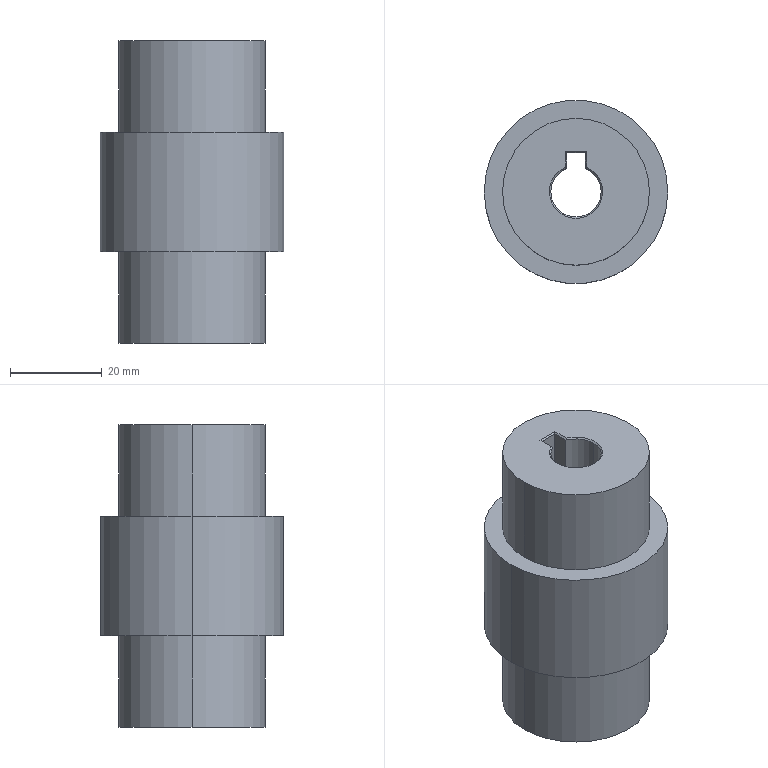Part | SolidWorks | features Cut 5, Boss 2, Chamfer 1, Extrusion 1 | 1 solid | 39 faces | box 40 x 40 x 66 mm | volume 50078 mm3 | plane 19 | cylinder 14 | cone 6 | commonest cylinder face diameters 32 x4 11 x3 19 x3 20 x2 40 x2
STEP:
#1=CARTESIAN_POINT('',(-5.5,0.,65.7));
#2=VERTEX_POINT('',#1);
#3=CARTESIAN_POINT('',(5.5,0.,65.7));
#4=VERTEX_POINT('',#3);
#5=CARTESIAN_POINT('',(0.,0.,65.7));
#6=DIRECTION('',(0.,0.,1.));
#7=DIRECTION('',(1.,0.,0.));
#8=AXIS2_PLACEMENT_3D('',#5,#6,#7);
#9=CIRCLE('',#8,5.5);
#10=EDGE_CURVE('',#2,#4,#9,.T.);
#11=ORIENTED_EDGE('',*,*,#10,.F.);
#12=CARTESIAN_POINT('',(-5.8,0.,66.));
#13=VERTEX_POINT('',#12);
#14=CARTESIAN_POINT('',(-5.5,0.,65.7));
#15=DIRECTION('',(-0.7071,0.,0.7071));
#16=VECTOR('',#15,1000.);
#17=LINE('',#14,#16);
#18=EDGE_CURVE('',#2,#13,#17,.T.);
#19=ORIENTED_EDGE('',*,*,#18,.T.);
#20=CARTESIAN_POINT('',(5.8,0.,66.));
#21=VERTEX_POINT('',#20);
#22=CARTESIAN_POINT('',(0.,0.,66.));
#23=DIRECTION('',(0.,0.,-1.));
#24=DIRECTION('',(1.,0.,0.));
#25=AXIS2_PLACEMENT_3D('',#22,#23,#24);
#26=CIRCLE('',#25,5.8);
#27=EDGE_CURVE('',#21,#13,#26,.T.);
#28=ORIENTED_EDGE('',*,*,#27,.F.);
#29=CARTESIAN_POINT('',(5.5,0.,65.7));
#30=DIRECTION('',(0.7071,0.,0.7071));
#31=VECTOR('',#30,1000.);
#32=LINE('',#29,#31);
#33=EDGE_CURVE('',#4,#21,#32,.T.);
#34=ORIENTED_EDGE('',*,*,#33,.F.);
#35=EDGE_LOOP('',(#11,#19,#28,#34));
#36=FACE_OUTER_BOUND('',#35,.T.);
#37=CARTESIAN_POINT('',(0.,0.,65.7));
#38=DIRECTION('',(0.,0.,1.));
#39=DIRECTION('',(1.,0.,0.));
#40=AXIS2_PLACEMENT_3D('',#37,#38,#39);
#41=CONICAL_SURFACE('',#40,5.5,0.7854);
#42=ADVANCED_FACE('',(#36),#41,.F.);
#43=CARTESIAN_POINT('',(2.,5.123,65.7));
#44=VERTEX_POINT('',#43);
#45=CARTESIAN_POINT('',(0.,0.,65.7));
#46=DIRECTION('',(0.,0.,1.));
#47=DIRECTION('',(1.,0.,0.));
#48=AXIS2_PLACEMENT_3D('',#45,#46,#47);
#49=CIRCLE('',#48,5.5);
#50=EDGE_CURVE('',#4,#44,#49,.T.);
#51=ORIENTED_EDGE('',*,*,#50,.F.);
#52=ORIENTED_EDGE('',*,*,#33,.T.);
#53=CARTESIAN_POINT('',(2.3,5.324,66.));
#54=VERTEX_POINT('',#53);
#55=CARTESIAN_POINT('',(0.,0.,66.));
#56=DIRECTION('',(0.,0.,-1.));
#57=DIRECTION('',(1.,0.,0.));
#58=AXIS2_PLACEMENT_3D('',#55,#56,#57);
#59=CIRCLE('',#58,5.8);
#60=EDGE_CURVE('',#54,#21,#59,.T.);
#61=ORIENTED_EDGE('',*,*,#60,.F.);
#62=CARTESIAN_POINT('',(2.,5.123,65.7));
#63=CARTESIAN_POINT('',(2.1,5.192,65.8));
#64=CARTESIAN_POINT('',(2.2,5.259,65.9));
#65=CARTESIAN_POINT('',(2.3,5.324,66.));
#66=B_SPLINE_CURVE_WITH_KNOTS('',3,(#62,#63,#64,#65),.UNSPECIFIED.,.F.,.F.,(4,4),(0.,0.0004695),.UNSPECIFIED.);
#67=EDGE_CURVE('',#44,#54,#66,.T.);
#68=ORIENTED_EDGE('',*,*,#67,.F.);
#69=EDGE_LOOP('',(#51,#52,#61,#68));
#70=FACE_OUTER_BOUND('',#69,.T.);
#71=CARTESIAN_POINT('',(0.,0.,65.7));
#72=DIRECTION('',(0.,0.,1.));
#73=DIRECTION('',(1.,0.,0.));
#74=AXIS2_PLACEMENT_3D('',#71,#72,#73);
#75=CONICAL_SURFACE('',#74,5.5,0.7854);
#76=ADVANCED_FACE('',(#70),#75,.F.);
#77=CARTESIAN_POINT('',(9.5,0.,0.3));
#78=VERTEX_POINT('',#77);
#79=CARTESIAN_POINT('',(-9.5,0.,0.3));
#80=VERTEX_POINT('',#79);
#81=CARTESIAN_POINT('',(0.,0.,0.3));
#82=DIRECTION('',(0.,0.,-1.));
#83=DIRECTION('',(1.,0.,0.));
#84=AXIS2_PLACEMENT_3D('',#81,#82,#83);
#85=CIRCLE('',#84,9.5);
#86=EDGE_CURVE('',#78,#80,#85,.T.);
#87=ORIENTED_EDGE('',*,*,#86,.F.);
#88=CARTESIAN_POINT('',(9.8,0.,0.));
#89=VERTEX_POINT('',#88);
#90=CARTESIAN_POINT('',(9.5,0.,0.3));
#91=DIRECTION('',(0.7071,0.,-0.7071));
#92=VECTOR('',#91,1000.);
#93=LINE('',#90,#92);
#94=EDGE_CURVE('',#78,#89,#93,.T.);
#95=ORIENTED_EDGE('',*,*,#94,.T.);
#96=CARTESIAN_POINT('',(-9.8,0.,0.));
#97=VERTEX_POINT('',#96);
#98=CARTESIAN_POINT('',(0.,0.,0.));
#99=DIRECTION('',(0.,0.,1.));
#100=DIRECTION('',(1.,0.,0.));
#101=AXIS2_PLACEMENT_3D('',#98,#99,#100);
#102=CIRCLE('',#101,9.8);
#103=EDGE_CURVE('',#97,#89,#102,.T.);
#104=ORIENTED_EDGE('',*,*,#103,.F.);
#105=CARTESIAN_POINT('',(-9.5,0.,0.3));
#106=DIRECTION('',(-0.7071,0.,-0.7071));
#107=VECTOR('',#106,1000.);
#108=LINE('',#105,#107);
#109=EDGE_CURVE('',#80,#97,#108,.T.);
#110=ORIENTED_EDGE('',*,*,#109,.F.);
#111=EDGE_LOOP('',(#87,#95,#104,#110));
#112=FACE_OUTER_BOUND('',#111,.T.);
#113=CARTESIAN_POINT('',(0.,0.,0.3));
#114=DIRECTION('',(0.,0.,-1.));
#115=DIRECTION('',(-1.,0.,0.));
#116=AXIS2_PLACEMENT_3D('',#113,#114,#115);
#117=CONICAL_SURFACE('',#116,9.5,0.7854);
#118=ADVANCED_FACE('',(#112),#117,.F.);
#119=CARTESIAN_POINT('',(-3.,9.014,0.3));
#120=VERTEX_POINT('',#119);
#121=CARTESIAN_POINT('',(0.,0.,0.3));
#122=DIRECTION('',(0.,0.,-1.));
#123=DIRECTION('',(1.,0.,0.));
#124=AXIS2_PLACEMENT_3D('',#121,#122,#123);
#125=CIRCLE('',#124,9.5);
#126=EDGE_CURVE('',#80,#120,#125,.T.);
#127=ORIENTED_EDGE('',*,*,#126,.F.);
#128=ORIENTED_EDGE('',*,*,#109,.T.);
#129=CARTESIAN_POINT('',(-3.3,9.228,0.));
#130=VERTEX_POINT('',#129);
#131=CARTESIAN_POINT('',(0.,0.,0.));
#132=DIRECTION('',(0.,0.,1.));
#133=DIRECTION('',(1.,0.,0.));
#134=AXIS2_PLACEMENT_3D('',#131,#132,#133);
#135=CIRCLE('',#134,9.8);
#136=EDGE_CURVE('',#130,#97,#135,.T.);
#137=ORIENTED_EDGE('',*,*,#136,.F.);
#138=CARTESIAN_POINT('',(-3.,9.014,0.3));
#139=CARTESIAN_POINT('',(-3.1,9.086,0.2002));
#140=CARTESIAN_POINT('',(-3.2,9.157,0.1002));
#141=CARTESIAN_POINT('',(-3.3,9.228,0.));
#142=B_SPLINE_CURVE_WITH_KNOTS('',3,(#138,#139,#140,#141),.UNSPECIFIED.,.F.,.F.,(4,4),(0.,0.0004751),.UNSPECIFIED.);
#143=EDGE_CURVE('',#120,#130,#142,.T.);
#144=ORIENTED_EDGE('',*,*,#143,.F.);
#145=EDGE_LOOP('',(#127,#128,#137,#144));
#146=FACE_OUTER_BOUND('',#145,.T.);
#147=CARTESIAN_POINT('',(0.,0.,0.3));
#148=DIRECTION('',(0.,0.,-1.));
#149=DIRECTION('',(-1.,0.,0.));
#150=AXIS2_PLACEMENT_3D('',#147,#148,#149);
#151=CONICAL_SURFACE('',#150,9.5,0.7854);
#152=ADVANCED_FACE('',(#146),#151,.F.);
#153=CARTESIAN_POINT('',(-10.,0.,27.));
#154=VERTEX_POINT('',#153);
#155=CARTESIAN_POINT('',(10.,0.,27.));
#156=VERTEX_POINT('',#155);
#157=CARTESIAN_POINT('',(0.,0.,27.));
#158=DIRECTION('',(0.,0.,1.));
#159=DIRECTION('',(1.,0.,0.));
#160=AXIS2_PLACEMENT_3D('',#157,#158,#159);
#161=CIRCLE('',#160,10.);
#162=EDGE_CURVE('',#154,#156,#161,.T.);
#163=ORIENTED_EDGE('',*,*,#162,.F.);
#164=CARTESIAN_POINT('',(-10.,0.,39.));
#165=VERTEX_POINT('',#164);
#166=CARTESIAN_POINT('',(-10.,0.,27.));
#167=DIRECTION('',(0.,0.,1.));
#168=VECTOR('',#167,1000.);
#169=LINE('',#166,#168);
#170=EDGE_CURVE('',#154,#165,#169,.T.);
#171=ORIENTED_EDGE('',*,*,#170,.T.);
#172=CARTESIAN_POINT('',(10.,0.,39.));
#173=VERTEX_POINT('',#172);
#174=CARTESIAN_POINT('',(0.,0.,39.));
#175=DIRECTION('',(0.,0.,1.));
#176=DIRECTION('',(1.,0.,0.));
#177=AXIS2_PLACEMENT_3D('',#174,#175,#176);
#178=CIRCLE('',#177,10.);
#179=EDGE_CURVE('',#165,#173,#178,.T.);
#180=ORIENTED_EDGE('',*,*,#179,.T.);
#181=CARTESIAN_POINT('',(10.,0.,27.));
#182=DIRECTION('',(0.,0.,1.));
#183=VECTOR('',#182,1000.);
#184=LINE('',#181,#183);
#185=EDGE_CURVE('',#156,#173,#184,.T.);
#186=ORIENTED_EDGE('',*,*,#185,.F.);
#187=EDGE_LOOP('',(#163,#171,#180,#186));
#188=FACE_OUTER_BOUND('',#187,.T.);
#189=CARTESIAN_POINT('',(0.,0.,27.));
#190=DIRECTION('',(0.,0.,1.));
#191=DIRECTION('',(1.,0.,0.));
#192=AXIS2_PLACEMENT_3D('',#189,#190,#191);
#193=CYLINDRICAL_SURFACE('',#192,10.);
#194=ADVANCED_FACE('',(#188),#193,.F.);
#195=CARTESIAN_POINT('',(5.5,0.,39.));
#196=VERTEX_POINT('',#195);
#197=CARTESIAN_POINT('',(-5.5,0.,39.));
#198=VERTEX_POINT('',#197);
#199=CARTESIAN_POINT('',(0.,0.,39.));
#200=DIRECTION('',(0.,0.,-1.));
#201=DIRECTION('',(1.,0.,0.));
#202=AXIS2_PLACEMENT_3D('',#199,#200,#201);
#203=CIRCLE('',#202,5.5);
#204=EDGE_CURVE('',#196,#198,#203,.T.);
#205=ORIENTED_EDGE('',*,*,#204,.T.);
#206=CARTESIAN_POINT('',(-5.5,0.,39.));
#207=DIRECTION('',(0.,0.,1.));
#208=VECTOR('',#207,1000.);
#209=LINE('',#206,#208);
#210=EDGE_CURVE('',#198,#2,#209,.T.);
#211=ORIENTED_EDGE('',*,*,#210,.T.);
#212=ORIENTED_EDGE('',*,*,#10,.T.);
#213=CARTESIAN_POINT('',(5.5,0.,39.));
#214=DIRECTION('',(0.,0.,1.));
#215=VECTOR('',#214,1000.);
#216=LINE('',#213,#215);
#217=EDGE_CURVE('',#196,#4,#216,.T.);
#218=ORIENTED_EDGE('',*,*,#217,.F.);
#219=EDGE_LOOP('',(#205,#211,#212,#218));
#220=FACE_OUTER_BOUND('',#219,.T.);
#221=CARTESIAN_POINT('',(0.,0.,39.));
#222=DIRECTION('',(0.,0.,1.));
#223=DIRECTION('',(1.,0.,0.));
#224=AXIS2_PLACEMENT_3D('',#221,#222,#223);
#225=CYLINDRICAL_SURFACE('',#224,5.5);
#226=ADVANCED_FACE('',(#220),#225,.F.);
#227=CARTESIAN_POINT('',(2.,5.123,39.));
#228=VERTEX_POINT('',#227);
#229=CARTESIAN_POINT('',(0.,0.,39.));
#230=DIRECTION('',(0.,0.,-1.));
#231=DIRECTION('',(1.,0.,0.));
#232=AXIS2_PLACEMENT_3D('',#229,#230,#231);
#233=CIRCLE('',#232,5.5);
#234=EDGE_CURVE('',#228,#196,#233,.T.);
#235=ORIENTED_EDGE('',*,*,#234,.T.);
#236=ORIENTED_EDGE('',*,*,#217,.T.);
#237=ORIENTED_EDGE('',*,*,#50,.T.);
#238=CARTESIAN_POINT('',(2.,5.123,39.));
#239=DIRECTION('',(0.,0.,1.));
#240=VECTOR('',#239,1000.);
#241=LINE('',#238,#240);
#242=EDGE_CURVE('',#228,#44,#241,.T.);
#243=ORIENTED_EDGE('',*,*,#242,.F.);
#244=EDGE_LOOP('',(#235,#236,#237,#243));
#245=FACE_OUTER_BOUND('',#244,.T.);
#246=CARTESIAN_POINT('',(0.,0.,39.));
#247=DIRECTION('',(0.,0.,1.));
#248=DIRECTION('',(1.,0.,0.));
#249=AXIS2_PLACEMENT_3D('',#246,#247,#248);
#250=CYLINDRICAL_SURFACE('',#249,5.5);
#251=ADVANCED_FACE('',(#245),#250,.F.);
#252=CARTESIAN_POINT('',(9.5,0.,27.));
#253=VERTEX_POINT('',#252);
#254=CARTESIAN_POINT('',(-9.5,0.,27.));
#255=VERTEX_POINT('',#254);
#256=CARTESIAN_POINT('',(0.,0.,27.));
#257=DIRECTION('',(0.,0.,-1.));
#258=DIRECTION('',(1.,0.,0.));
#259=AXIS2_PLACEMENT_3D('',#256,#257,#258);
#260=CIRCLE('',#259,9.5);
#261=EDGE_CURVE('',#253,#255,#260,.T.);
#262=ORIENTED_EDGE('',*,*,#261,.F.);
#263=CARTESIAN_POINT('',(9.5,0.,27.));
#264=DIRECTION('',(0.,0.,-1.));
#265=VECTOR('',#264,1000.);
#266=LINE('',#263,#265);
#267=EDGE_CURVE('',#253,#78,#266,.T.);
#268=ORIENTED_EDGE('',*,*,#267,.T.);
#269=ORIENTED_EDGE('',*,*,#86,.T.);
#270=CARTESIAN_POINT('',(-9.5,0.,27.));
#271=DIRECTION('',(0.,0.,-1.));
#272=VECTOR('',#271,1000.);
#273=LINE('',#270,#272);
#274=EDGE_CURVE('',#255,#80,#273,.T.);
#275=ORIENTED_EDGE('',*,*,#274,.F.);
#276=EDGE_LOOP('',(#262,#268,#269,#275));
#277=FACE_OUTER_BOUND('',#276,.T.);
#278=CARTESIAN_POINT('',(0.,0.,27.));
#279=DIRECTION('',(0.,0.,-1.));
#280=DIRECTION('',(-1.,0.,0.));
#281=AXIS2_PLACEMENT_3D('',#278,#279,#280);
#282=CYLINDRICAL_SURFACE('',#281,9.5);
#283=ADVANCED_FACE('',(#277),#282,.F.);
#284=CARTESIAN_POINT('',(-3.,9.014,27.));
#285=VERTEX_POINT('',#284);
#286=CARTESIAN_POINT('',(0.,0.,27.));
#287=DIRECTION('',(0.,0.,-1.));
#288=DIRECTION('',(1.,0.,0.));
#289=AXIS2_PLACEMENT_3D('',#286,#287,#288);
#290=CIRCLE('',#289,9.5);
#291=EDGE_CURVE('',#255,#285,#290,.T.);
#292=ORIENTED_EDGE('',*,*,#291,.F.);
#293=ORIENTED_EDGE('',*,*,#274,.T.);
#294=ORIENTED_EDGE('',*,*,#126,.T.);
#295=CARTESIAN_POINT('',(-3.,9.014,27.));
#296=DIRECTION('',(0.,0.,-1.));
#297=VECTOR('',#296,1000.);
#298=LINE('',#295,#297);
#299=EDGE_CURVE('',#285,#120,#298,.T.);
#300=ORIENTED_EDGE('',*,*,#299,.F.);
#301=EDGE_LOOP('',(#292,#293,#294,#300));
#302=FACE_OUTER_BOUND('',#301,.T.);
#303=CARTESIAN_POINT('',(0.,0.,27.));
#304=DIRECTION('',(0.,0.,-1.));
#305=DIRECTION('',(-1.,0.,0.));
#306=AXIS2_PLACEMENT_3D('',#303,#304,#305);
#307=CYLINDRICAL_SURFACE('',#306,9.5);
#308=ADVANCED_FACE('',(#302),#307,.F.);
#309=CARTESIAN_POINT('',(16.,0.,66.));
#310=VERTEX_POINT('',#309);
#311=CARTESIAN_POINT('',(-16.,0.,66.));
#312=VERTEX_POINT('',#311);
#313=CARTESIAN_POINT('',(0.,0.,66.));
#314=DIRECTION('',(0.,0.,1.));
#315=DIRECTION('',(1.,0.,0.));
#316=AXIS2_PLACEMENT_3D('',#313,#314,#315);
#317=CIRCLE('',#316,16.);
#318=EDGE_CURVE('',#310,#312,#317,.T.);
#319=ORIENTED_EDGE('',*,*,#318,.F.);
#320=CARTESIAN_POINT('',(16.,0.,46.));
#321=VERTEX_POINT('',#320);
#322=CARTESIAN_POINT('',(16.,0.,66.));
#323=DIRECTION('',(0.,0.,-1.));
#324=VECTOR('',#323,1000.);
#325=LINE('',#322,#324);
#326=EDGE_CURVE('',#310,#321,#325,.T.);
#327=ORIENTED_EDGE('',*,*,#326,.T.);
#328=CARTESIAN_POINT('',(-16.,0.,46.));
#329=VERTEX_POINT('',#328);
#330=CARTESIAN_POINT('',(0.,0.,46.));
#331=DIRECTION('',(0.,0.,1.));
#332=DIRECTION('',(1.,0.,0.));
#333=AXIS2_PLACEMENT_3D('',#330,#331,#332);
#334=CIRCLE('',#333,16.);
#335=EDGE_CURVE('',#321,#329,#334,.T.);
#336=ORIENTED_EDGE('',*,*,#335,.T.);
#337=CARTESIAN_POINT('',(-16.,0.,66.));
#338=DIRECTION('',(0.,0.,-1.));
#339=VECTOR('',#338,1000.);
#340=LINE('',#337,#339);
#341=EDGE_CURVE('',#312,#329,#340,.T.);
#342=ORIENTED_EDGE('',*,*,#341,.F.);
#343=EDGE_LOOP('',(#319,#327,#336,#342));
#344=FACE_OUTER_BOUND('',#343,.T.);
#345=CARTESIAN_POINT('',(0.,0.,66.));
#346=DIRECTION('',(0.,0.,-1.));
#347=DIRECTION('',(-1.,0.,0.));
#348=AXIS2_PLACEMENT_3D('',#345,#346,#347);
#349=CYLINDRICAL_SURFACE('',#348,16.);
#350=ADVANCED_FACE('',(#344),#349,.T.);
#351=CARTESIAN_POINT('',(20.,0.,46.));
#352=VERTEX_POINT('',#351);
#353=CARTESIAN_POINT('',(-20.,0.,46.));
#354=VERTEX_POINT('',#353);
#355=CARTESIAN_POINT('',(0.,0.,46.));
#356=DIRECTION('',(0.,0.,1.));
#357=DIRECTION('',(1.,0.,0.));
#358=AXIS2_PLACEMENT_3D('',#355,#356,#357);
#359=CIRCLE('',#358,20.);
#360=EDGE_CURVE('',#352,#354,#359,.T.);
#361=ORIENTED_EDGE('',*,*,#360,.F.);
#362=CARTESIAN_POINT('',(20.,0.,20.));
#363=VERTEX_POINT('',#362);
#364=CARTESIAN_POINT('',(20.,0.,46.));
#365=DIRECTION('',(0.,0.,-1.));
#366=VECTOR('',#365,1000.);
#367=LINE('',#364,#366);
#368=EDGE_CURVE('',#352,#363,#367,.T.);
#369=ORIENTED_EDGE('',*,*,#368,.T.);
#370=CARTESIAN_POINT('',(-20.,0.,20.));
#371=VERTEX_POINT('',#370);
#372=CARTESIAN_POINT('',(0.,0.,20.));
#373=DIRECTION('',(0.,0.,1.));
#374=DIRECTION('',(1.,0.,0.));
#375=AXIS2_PLACEMENT_3D('',#372,#373,#374);
#376=CIRCLE('',#375,20.);
#377=EDGE_CURVE('',#363,#371,#376,.T.);
#378=ORIENTED_EDGE('',*,*,#377,.T.);
#379=CARTESIAN_POINT('',(-20.,0.,46.));
#380=DIRECTION('',(0.,0.,-1.));
#381=VECTOR('',#380,1000.);
#382=LINE('',#379,#381);
#383=EDGE_CURVE('',#354,#371,#382,.T.);
#384=ORIENTED_EDGE('',*,*,#383,.F.);
#385=EDGE_LOOP('',(#361,#369,#378,#384));
#386=FACE_OUTER_BOUND('',#385,.T.);
#387=CARTESIAN_POINT('',(0.,0.,46.));
#388=DIRECTION('',(0.,0.,-1.));
#389=DIRECTION('',(-1.,0.,0.));
#390=AXIS2_PLACEMENT_3D('',#387,#388,#389);
#391=CYLINDRICAL_SURFACE('',#390,20.);
#392=ADVANCED_FACE('',(#386),#391,.T.);
#393=CARTESIAN_POINT('',(16.,0.,20.));
#394=VERTEX_POINT('',#393);
#395=CARTESIAN_POINT('',(-16.,0.,20.));
#396=VERTEX_POINT('',#395);
#397=CARTESIAN_POINT('',(0.,0.,20.));
#398=DIRECTION('',(0.,0.,1.));
#399=DIRECTION('',(1.,0.,0.));
#400=AXIS2_PLACEMENT_3D('',#397,#398,#399);
#401=CIRCLE('',#400,16.);
#402=EDGE_CURVE('',#394,#396,#401,.T.);
#403=ORIENTED_EDGE('',*,*,#402,.F.);
#404=CARTESIAN_POINT('',(16.,0.,0.));
#405=VERTEX_POINT('',#404);
#406=CARTESIAN_POINT('',(16.,0.,20.));
#407=DIRECTION('',(0.,0.,-1.));
#408=VECTOR('',#407,1000.);
#409=LINE('',#406,#408);
#410=EDGE_CURVE('',#394,#405,#409,.T.);
#411=ORIENTED_EDGE('',*,*,#410,.T.);
#412=CARTESIAN_POINT('',(-16.,0.,0.));
#413=VERTEX_POINT('',#412);
#414=CARTESIAN_POINT('',(0.,0.,0.));
#415=DIRECTION('',(0.,0.,1.));
#416=DIRECTION('',(1.,0.,0.));
#417=AXIS2_PLACEMENT_3D('',#414,#415,#416);
#418=CIRCLE('',#417,16.);
#419=EDGE_CURVE('',#405,#413,#418,.T.);
#420=ORIENTED_EDGE('',*,*,#419,.T.);
#421=CARTESIAN_POINT('',(-16.,0.,20.));
#422=DIRECTION('',(0.,0.,-1.));
#423=VECTOR('',#422,1000.);
#424=LINE('',#421,#423);
#425=EDGE_CURVE('',#396,#413,#424,.T.);
#426=ORIENTED_EDGE('',*,*,#425,.F.);
#427=EDGE_LOOP('',(#403,#411,#420,#426));
#428=FACE_OUTER_BOUND('',#427,.T.);
#429=CARTESIAN_POINT('',(0.,0.,20.));
#430=DIRECTION('',(0.,0.,-1.));
#431=DIRECTION('',(-1.,0.,0.));
#432=AXIS2_PLACEMENT_3D('',#429,#430,#431);
#433=CYLINDRICAL_SURFACE('',#432,16.);
#434=ADVANCED_FACE('',(#428),#433,.T.);
#435=CARTESIAN_POINT('',(0.,0.,46.));
#436=DIRECTION('',(0.,0.,1.));
#437=DIRECTION('',(1.,0.,0.));
#438=AXIS2_PLACEMENT_3D('',#435,#436,#437);
#439=CIRCLE('',#438,20.);
#440=EDGE_CURVE('',#354,#352,#439,.T.);
#441=ORIENTED_EDGE('',*,*,#440,.T.);
#442=ORIENTED_EDGE('',*,*,#360,.T.);
#443=EDGE_LOOP('',(#441,#442));
#444=FACE_OUTER_BOUND('',#443,.T.);
#445=CARTESIAN_POINT('',(0.,0.,46.));
#446=DIRECTION('',(0.,0.,1.));
#447=DIRECTION('',(1.,0.,0.));
#448=AXIS2_PLACEMENT_3D('',#445,#446,#447);
#449=CIRCLE('',#448,16.);
#450=EDGE_CURVE('',#329,#321,#449,.T.);
#451=ORIENTED_EDGE('',*,*,#450,.F.);
#452=ORIENTED_EDGE('',*,*,#335,.F.);
#453=EDGE_LOOP('',(#451,#452));
#454=FACE_BOUND('',#453,.T.);
#455=CARTESIAN_POINT('',(0.,0.,46.));
#456=DIRECTION('',(0.,0.,1.));
#457=DIRECTION('',(1.,0.,0.));
#458=AXIS2_PLACEMENT_3D('',#455,#456,#457);
#459=PLANE('',#458);
#460=ADVANCED_FACE('',(#444,#454),#459,.T.);
#461=ORIENTED_EDGE('',*,*,#410,.F.);
#462=CARTESIAN_POINT('',(0.,0.,20.));
#463=DIRECTION('',(0.,0.,1.));
#464=DIRECTION('',(1.,0.,0.));
#465=AXIS2_PLACEMENT_3D('',#462,#463,#464);
#466=CIRCLE('',#465,16.);
#467=EDGE_CURVE('',#396,#394,#466,.T.);
#468=ORIENTED_EDGE('',*,*,#467,.F.);
#469=ORIENTED_EDGE('',*,*,#425,.T.);
#470=CARTESIAN_POINT('',(0.,0.,0.));
#471=DIRECTION('',(0.,0.,1.));
#472=DIRECTION('',(1.,0.,0.));
#473=AXIS2_PLACEMENT_3D('',#470,#471,#472);
#474=CIRCLE('',#473,16.);
#475=EDGE_CURVE('',#413,#405,#474,.T.);
#476=ORIENTED_EDGE('',*,*,#475,.T.);
#477=EDGE_LOOP('',(#461,#468,#469,#476));
#478=FACE_OUTER_BOUND('',#477,.T.);
#479=CARTESIAN_POINT('',(0.,0.,20.));
#480=DIRECTION('',(0.,0.,-1.));
#481=DIRECTION('',(-1.,0.,0.));
#482=AXIS2_PLACEMENT_3D('',#479,#480,#481);
#483=CYLINDRICAL_SURFACE('',#482,16.);
#484=ADVANCED_FACE('',(#478),#483,.T.);
#485=CARTESIAN_POINT('',(3.3,12.3,0.));
#486=VERTEX_POINT('',#485);
#487=CARTESIAN_POINT('',(-3.3,12.3,0.));
#488=VERTEX_POINT('',#487);
#489=CARTESIAN_POINT('',(0.,12.3,0.));
#490=DIRECTION('',(-1.,0.,0.));
#491=VECTOR('',#490,1000.);
#492=LINE('',#489,#491);
#493=EDGE_CURVE('',#486,#488,#492,.T.);
#494=ORIENTED_EDGE('',*,*,#493,.T.);
#495=CARTESIAN_POINT('',(-3.3,0.,0.));
#496=DIRECTION('',(0.,-1.,0.));
#497=VECTOR('',#496,1000.);
#498=LINE('',#495,#497);
#499=EDGE_CURVE('',#488,#130,#498,.T.);
#500=ORIENTED_EDGE('',*,*,#499,.T.);
#501=ORIENTED_EDGE('',*,*,#136,.T.);
#502=ORIENTED_EDGE('',*,*,#103,.T.);
#503=CARTESIAN_POINT('',(3.3,9.228,0.));
#504=VERTEX_POINT('',#503);
#505=CARTESIAN_POINT('',(0.,0.,0.));
#506=DIRECTION('',(0.,0.,1.));
#507=DIRECTION('',(1.,0.,0.));
#508=AXIS2_PLACEMENT_3D('',#505,#506,#507);
#509=CIRCLE('',#508,9.8);
#510=EDGE_CURVE('',#89,#504,#509,.T.);
#511=ORIENTED_EDGE('',*,*,#510,.T.);
#512=CARTESIAN_POINT('',(3.3,0.,0.));
#513=DIRECTION('',(0.,1.,0.));
#514=VECTOR('',#513,1000.);
#515=LINE('',#512,#514);
#516=EDGE_CURVE('',#504,#486,#515,.T.);
#517=ORIENTED_EDGE('',*,*,#516,.T.);
#518=EDGE_LOOP('',(#494,#500,#501,#502,#511,#517));
#519=FACE_BOUND('',#518,.T.);
#520=ORIENTED_EDGE('',*,*,#475,.F.);
#521=ORIENTED_EDGE('',*,*,#419,.F.);
#522=EDGE_LOOP('',(#520,#521));
#523=FACE_OUTER_BOUND('',#522,.T.);
#524=CARTESIAN_POINT('',(0.,0.,0.));
#525=DIRECTION('',(0.,0.,1.));
#526=DIRECTION('',(1.,0.,0.));
#527=AXIS2_PLACEMENT_3D('',#524,#525,#526);
#528=PLANE('',#527);
#529=ADVANCED_FACE('',(#519,#523),#528,.F.);
#530=CARTESIAN_POINT('',(0.,0.,20.));
#531=DIRECTION('',(0.,0.,1.));
#532=DIRECTION('',(1.,0.,0.));
#533=AXIS2_PLACEMENT_3D('',#530,#531,#532);
#534=CIRCLE('',#533,20.);
#535=EDGE_CURVE('',#371,#363,#534,.T.);
#536=ORIENTED_EDGE('',*,*,#535,.F.);
#537=ORIENTED_EDGE('',*,*,#377,.F.);
#538=EDGE_LOOP('',(#536,#537));
#539=FACE_OUTER_BOUND('',#538,.T.);
#540=ORIENTED_EDGE('',*,*,#467,.T.);
#541=ORIENTED_EDGE('',*,*,#402,.T.);
#542=EDGE_LOOP('',(#540,#541));
#543=FACE_BOUND('',#542,.T.);
#544=CARTESIAN_POINT('',(0.,0.,20.));
#545=DIRECTION('',(0.,0.,1.));
#546=DIRECTION('',(1.,0.,0.));
#547=AXIS2_PLACEMENT_3D('',#544,#545,#546);
#548=PLANE('',#547);
#549=ADVANCED_FACE('',(#539,#543),#548,.F.);
#550=ORIENTED_EDGE('',*,*,#368,.F.);
#551=ORIENTED_EDGE('',*,*,#440,.F.);
#552=ORIENTED_EDGE('',*,*,#383,.T.);
#553=ORIENTED_EDGE('',*,*,#535,.T.);
#554=EDGE_LOOP('',(#550,#551,#552,#553));
#555=FACE_OUTER_BOUND('',#554,.T.);
#556=CARTESIAN_POINT('',(0.,0.,46.));
#557=DIRECTION('',(0.,0.,-1.));
#558=DIRECTION('',(-1.,0.,0.));
#559=AXIS2_PLACEMENT_3D('',#556,#557,#558);
#560=CYLINDRICAL_SURFACE('',#559,20.);
#561=ADVANCED_FACE('',(#555),#560,.T.);
#562=ORIENTED_EDGE('',*,*,#326,.F.);
#563=CARTESIAN_POINT('',(0.,0.,66.));
#564=DIRECTION('',(0.,0.,1.));
#565=DIRECTION('',(1.,0.,0.));
#566=AXIS2_PLACEMENT_3D('',#563,#564,#565);
#567=CIRCLE('',#566,16.);
#568=EDGE_CURVE('',#312,#310,#567,.T.);
#569=ORIENTED_EDGE('',*,*,#568,.F.);
#570=ORIENTED_EDGE('',*,*,#341,.T.);
#571=ORIENTED_EDGE('',*,*,#450,.T.);
#572=EDGE_LOOP('',(#562,#569,#570,#571));
#573=FACE_OUTER_BOUND('',#572,.T.);
#574=CARTESIAN_POINT('',(0.,0.,66.));
#575=DIRECTION('',(0.,0.,-1.));
#576=DIRECTION('',(-1.,0.,0.));
#577=AXIS2_PLACEMENT_3D('',#574,#575,#576);
#578=CYLINDRICAL_SURFACE('',#577,16.);
#579=ADVANCED_FACE('',(#573),#578,.T.);
#580=CARTESIAN_POINT('',(-2.3,8.8,66.));
#581=VERTEX_POINT('',#580);
#582=CARTESIAN_POINT('',(2.3,8.8,66.));
#583=VERTEX_POINT('',#582);
#584=CARTESIAN_POINT('',(2.,8.8,66.));
#585=DIRECTION('',(1.,0.,0.));
#586=VECTOR('',#585,1000.);
#587=LINE('',#584,#586);
#588=EDGE_CURVE('',#581,#583,#587,.T.);
#589=ORIENTED_EDGE('',*,*,#588,.T.);
#590=CARTESIAN_POINT('',(2.3,5.123,66.));
#591=DIRECTION('',(0.,-1.,0.));
#592=VECTOR('',#591,1000.);
#593=LINE('',#590,#592);
#594=EDGE_CURVE('',#583,#54,#593,.T.);
#595=ORIENTED_EDGE('',*,*,#594,.T.);
#596=ORIENTED_EDGE('',*,*,#60,.T.);
#597=ORIENTED_EDGE('',*,*,#27,.T.);
#598=CARTESIAN_POINT('',(-2.3,5.324,66.));
#599=VERTEX_POINT('',#598);
#600=CARTESIAN_POINT('',(0.,0.,66.));
#601=DIRECTION('',(0.,0.,-1.));
#602=DIRECTION('',(1.,0.,0.));
#603=AXIS2_PLACEMENT_3D('',#600,#601,#602);
#604=CIRCLE('',#603,5.8);
#605=EDGE_CURVE('',#13,#599,#604,.T.);
#606=ORIENTED_EDGE('',*,*,#605,.T.);
#607=CARTESIAN_POINT('',(-2.3,8.5,66.));
#608=DIRECTION('',(0.,1.,0.));
#609=VECTOR('',#608,1000.);
#610=LINE('',#607,#609);
#611=EDGE_CURVE('',#599,#581,#610,.T.);
#612=ORIENTED_EDGE('',*,*,#611,.T.);
#613=EDGE_LOOP('',(#589,#595,#596,#597,#606,#612));
#614=FACE_BOUND('',#613,.T.);
#615=ORIENTED_EDGE('',*,*,#568,.T.);
#616=ORIENTED_EDGE('',*,*,#318,.T.);
#617=EDGE_LOOP('',(#615,#616));
#618=FACE_OUTER_BOUND('',#617,.T.);
#619=CARTESIAN_POINT('',(0.,0.,66.));
#620=DIRECTION('',(0.,0.,1.));
#621=DIRECTION('',(1.,0.,0.));
#622=AXIS2_PLACEMENT_3D('',#619,#620,#621);
#623=PLANE('',#622);
#624=ADVANCED_FACE('',(#614,#618),#623,.T.);
#625=ORIENTED_EDGE('',*,*,#267,.F.);
#626=CARTESIAN_POINT('',(3.,9.014,27.));
#627=VERTEX_POINT('',#626);
#628=CARTESIAN_POINT('',(0.,0.,27.));
#629=DIRECTION('',(0.,0.,-1.));
#630=DIRECTION('',(1.,0.,0.));
#631=AXIS2_PLACEMENT_3D('',#628,#629,#630);
#632=CIRCLE('',#631,9.5);
#633=EDGE_CURVE('',#627,#253,#632,.T.);
#634=ORIENTED_EDGE('',*,*,#633,.F.);
#635=CARTESIAN_POINT('',(3.,9.014,0.3));
#636=VERTEX_POINT('',#635);
#637=CARTESIAN_POINT('',(3.,9.014,27.));
#638=DIRECTION('',(0.,0.,-1.));
#639=VECTOR('',#638,1000.);
#640=LINE('',#637,#639);
#641=EDGE_CURVE('',#627,#636,#640,.T.);
#642=ORIENTED_EDGE('',*,*,#641,.T.);
#643=CARTESIAN_POINT('',(0.,0.,0.3));
#644=DIRECTION('',(0.,0.,-1.));
#645=DIRECTION('',(1.,0.,0.));
#646=AXIS2_PLACEMENT_3D('',#643,#644,#645);
#647=CIRCLE('',#646,9.5);
#648=EDGE_CURVE('',#636,#78,#647,.T.);
#649=ORIENTED_EDGE('',*,*,#648,.T.);
#650=EDGE_LOOP('',(#625,#634,#642,#649));
#651=FACE_OUTER_BOUND('',#650,.T.);
#652=CARTESIAN_POINT('',(0.,0.,27.));
#653=DIRECTION('',(0.,0.,-1.));
#654=DIRECTION('',(-1.,0.,0.));
#655=AXIS2_PLACEMENT_3D('',#652,#653,#654);
#656=CYLINDRICAL_SURFACE('',#655,9.5);
#657=ADVANCED_FACE('',(#651),#656,.F.);
#658=ORIENTED_EDGE('',*,*,#210,.F.);
#659=CARTESIAN_POINT('',(-2.,5.123,39.));
#660=VERTEX_POINT('',#659);
#661=CARTESIAN_POINT('',(0.,0.,39.));
#662=DIRECTION('',(0.,0.,-1.));
#663=DIRECTION('',(1.,0.,0.));
#664=AXIS2_PLACEMENT_3D('',#661,#662,#663);
#665=CIRCLE('',#664,5.5);
#666=EDGE_CURVE('',#198,#660,#665,.T.);
#667=ORIENTED_EDGE('',*,*,#666,.T.);
#668=CARTESIAN_POINT('',(-2.,5.123,65.7));
#669=VERTEX_POINT('',#668);
#670=CARTESIAN_POINT('',(-2.,5.123,39.));
#671=DIRECTION('',(0.,0.,1.));
#672=VECTOR('',#671,1000.);
#673=LINE('',#670,#672);
#674=EDGE_CURVE('',#660,#669,#673,.T.);
#675=ORIENTED_EDGE('',*,*,#674,.T.);
#676=CARTESIAN_POINT('',(0.,0.,65.7));
#677=DIRECTION('',(0.,0.,1.));
#678=DIRECTION('',(1.,0.,0.));
#679=AXIS2_PLACEMENT_3D('',#676,#677,#678);
#680=CIRCLE('',#679,5.5);
#681=EDGE_CURVE('',#669,#2,#680,.T.);
#682=ORIENTED_EDGE('',*,*,#681,.T.);
#683=EDGE_LOOP('',(#658,#667,#675,#682));
#684=FACE_OUTER_BOUND('',#683,.T.);
#685=CARTESIAN_POINT('',(0.,0.,39.));
#686=DIRECTION('',(0.,0.,1.));
#687=DIRECTION('',(1.,0.,0.));
#688=AXIS2_PLACEMENT_3D('',#685,#686,#687);
#689=CYLINDRICAL_SURFACE('',#688,5.5);
#690=ADVANCED_FACE('',(#684),#689,.F.);
#691=CARTESIAN_POINT('',(-3.,9.539,27.));
#692=VERTEX_POINT('',#691);
#693=CARTESIAN_POINT('',(-3.,12.,27.));
#694=DIRECTION('',(0.,1.,0.));
#695=VECTOR('',#694,1000.);
#696=LINE('',#693,#695);
#697=EDGE_CURVE('',#285,#692,#696,.T.);
#698=ORIENTED_EDGE('',*,*,#697,.T.);
#699=CARTESIAN_POINT('',(0.,0.,27.));
#700=DIRECTION('',(0.,0.,1.));
#701=DIRECTION('',(1.,0.,0.));
#702=AXIS2_PLACEMENT_3D('',#699,#700,#701);
#703=CIRCLE('',#702,10.);
#704=EDGE_CURVE('',#692,#154,#703,.T.);
#705=ORIENTED_EDGE('',*,*,#704,.T.);
#706=ORIENTED_EDGE('',*,*,#162,.T.);
#707=CARTESIAN_POINT('',(3.,9.539,27.));
#708=VERTEX_POINT('',#707);
#709=CARTESIAN_POINT('',(0.,0.,27.));
#710=DIRECTION('',(0.,0.,1.));
#711=DIRECTION('',(1.,0.,0.));
#712=AXIS2_PLACEMENT_3D('',#709,#710,#711);
#713=CIRCLE('',#712,10.);
#714=EDGE_CURVE('',#156,#708,#713,.T.);
#715=ORIENTED_EDGE('',*,*,#714,.T.);
#716=CARTESIAN_POINT('',(3.,12.,27.));
#717=DIRECTION('',(0.,-1.,0.));
#718=VECTOR('',#717,1000.);
#719=LINE('',#716,#718);
#720=EDGE_CURVE('',#708,#627,#719,.T.);
#721=ORIENTED_EDGE('',*,*,#720,.T.);
#722=ORIENTED_EDGE('',*,*,#633,.T.);
#723=ORIENTED_EDGE('',*,*,#261,.T.);
#724=ORIENTED_EDGE('',*,*,#291,.T.);
#725=EDGE_LOOP('',(#698,#705,#706,#715,#721,#722,#723,#724));
#726=FACE_OUTER_BOUND('',#725,.T.);
#727=CARTESIAN_POINT('',(0.,0.,27.));
#728=DIRECTION('',(0.,0.,1.));
#729=DIRECTION('',(1.,0.,0.));
#730=AXIS2_PLACEMENT_3D('',#727,#728,#729);
#731=PLANE('',#730);
#732=ADVANCED_FACE('',(#726),#731,.T.);
#733=CARTESIAN_POINT('',(0.,0.,39.));
#734=DIRECTION('',(0.,0.,1.));
#735=DIRECTION('',(1.,0.,0.));
#736=AXIS2_PLACEMENT_3D('',#733,#734,#735);
#737=CIRCLE('',#736,10.);
#738=EDGE_CURVE('',#173,#165,#737,.T.);
#739=ORIENTED_EDGE('',*,*,#738,.F.);
#740=ORIENTED_EDGE('',*,*,#179,.F.);
#741=EDGE_LOOP('',(#739,#740));
#742=FACE_OUTER_BOUND('',#741,.T.);
#743=ORIENTED_EDGE('',*,*,#234,.F.);
#744=CARTESIAN_POINT('',(2.,8.5,39.));
#745=VERTEX_POINT('',#744);
#746=CARTESIAN_POINT('',(2.,8.5,39.));
#747=DIRECTION('',(0.,1.,0.));
#748=VECTOR('',#747,1000.);
#749=LINE('',#746,#748);
#750=EDGE_CURVE('',#228,#745,#749,.T.);
#751=ORIENTED_EDGE('',*,*,#750,.T.);
#752=CARTESIAN_POINT('',(-2.,8.5,39.));
#753=VERTEX_POINT('',#752);
#754=CARTESIAN_POINT('',(-2.,8.5,39.));
#755=DIRECTION('',(-1.,0.,0.));
#756=VECTOR('',#755,1000.);
#757=LINE('',#754,#756);
#758=EDGE_CURVE('',#745,#753,#757,.T.);
#759=ORIENTED_EDGE('',*,*,#758,.T.);
#760=CARTESIAN_POINT('',(-2.,8.5,39.));
#761=DIRECTION('',(0.,-1.,0.));
#762=VECTOR('',#761,1000.);
#763=LINE('',#760,#762);
#764=EDGE_CURVE('',#753,#660,#763,.T.);
#765=ORIENTED_EDGE('',*,*,#764,.T.);
#766=ORIENTED_EDGE('',*,*,#666,.F.);
#767=ORIENTED_EDGE('',*,*,#204,.F.);
#768=EDGE_LOOP('',(#743,#751,#759,#765,#766,#767));
#769=FACE_BOUND('',#768,.T.);
#770=CARTESIAN_POINT('',(0.,0.,39.));
#771=DIRECTION('',(0.,0.,1.));
#772=DIRECTION('',(1.,0.,0.));
#773=AXIS2_PLACEMENT_3D('',#770,#771,#772);
#774=PLANE('',#773);
#775=ADVANCED_FACE('',(#742,#769),#774,.F.);
#776=ORIENTED_EDGE('',*,*,#170,.F.);
#777=ORIENTED_EDGE('',*,*,#704,.F.);
#778=CARTESIAN_POINT('',(0.,0.,27.));
#779=DIRECTION('',(0.,0.,1.));
#780=DIRECTION('',(1.,0.,0.));
#781=AXIS2_PLACEMENT_3D('',#778,#779,#780);
#782=CIRCLE('',#781,10.);
#783=EDGE_CURVE('',#708,#692,#782,.T.);
#784=ORIENTED_EDGE('',*,*,#783,.F.);
#785=ORIENTED_EDGE('',*,*,#714,.F.);
#786=ORIENTED_EDGE('',*,*,#185,.T.);
#787=ORIENTED_EDGE('',*,*,#738,.T.);
#788=EDGE_LOOP('',(#776,#777,#784,#785,#786,#787));
#789=FACE_OUTER_BOUND('',#788,.T.);
#790=CARTESIAN_POINT('',(0.,0.,27.));
#791=DIRECTION('',(0.,0.,1.));
#792=DIRECTION('',(1.,0.,0.));
#793=AXIS2_PLACEMENT_3D('',#790,#791,#792);
#794=CYLINDRICAL_SURFACE('',#793,10.);
#795=ADVANCED_FACE('',(#789),#794,.F.);
#796=ORIENTED_EDGE('',*,*,#783,.T.);
#797=CARTESIAN_POINT('',(-3.,12.,27.));
#798=VERTEX_POINT('',#797);
#799=CARTESIAN_POINT('',(-3.,12.,27.));
#800=DIRECTION('',(0.,1.,0.));
#801=VECTOR('',#800,1000.);
#802=LINE('',#799,#801);
#803=EDGE_CURVE('',#692,#798,#802,.T.);
#804=ORIENTED_EDGE('',*,*,#803,.T.);
#805=CARTESIAN_POINT('',(3.,12.,27.));
#806=VERTEX_POINT('',#805);
#807=CARTESIAN_POINT('',(3.,12.,27.));
#808=DIRECTION('',(1.,0.,0.));
#809=VECTOR('',#808,1000.);
#810=LINE('',#807,#809);
#811=EDGE_CURVE('',#798,#806,#810,.T.);
#812=ORIENTED_EDGE('',*,*,#811,.T.);
#813=CARTESIAN_POINT('',(3.,12.,27.));
#814=DIRECTION('',(0.,-1.,0.));
#815=VECTOR('',#814,1000.);
#816=LINE('',#813,#815);
#817=EDGE_CURVE('',#806,#708,#816,.T.);
#818=ORIENTED_EDGE('',*,*,#817,.T.);
#819=EDGE_LOOP('',(#796,#804,#812,#818));
#820=FACE_OUTER_BOUND('',#819,.T.);
#821=CARTESIAN_POINT('',(0.,0.,27.));
#822=DIRECTION('',(0.,0.,-1.));
#823=DIRECTION('',(-1.,0.,0.));
#824=AXIS2_PLACEMENT_3D('',#821,#822,#823);
#825=PLANE('',#824);
#826=ADVANCED_FACE('',(#820),#825,.T.);
#827=CARTESIAN_POINT('',(-3.,12.,0.3));
#828=VERTEX_POINT('',#827);
#829=CARTESIAN_POINT('',(-3.,12.,27.));
#830=DIRECTION('',(0.,0.,-1.));
#831=VECTOR('',#830,1000.);
#832=LINE('',#829,#831);
#833=EDGE_CURVE('',#798,#828,#832,.T.);
#834=ORIENTED_EDGE('',*,*,#833,.T.);
#835=CARTESIAN_POINT('',(3.,12.,0.3));
#836=VERTEX_POINT('',#835);
#837=CARTESIAN_POINT('',(3.,12.,0.3));
#838=DIRECTION('',(1.,0.,0.));
#839=VECTOR('',#838,1000.);
#840=LINE('',#837,#839);
#841=EDGE_CURVE('',#828,#836,#840,.T.);
#842=ORIENTED_EDGE('',*,*,#841,.T.);
#843=CARTESIAN_POINT('',(3.,12.,27.));
#844=DIRECTION('',(0.,0.,-1.));
#845=VECTOR('',#844,1000.);
#846=LINE('',#843,#845);
#847=EDGE_CURVE('',#806,#836,#846,.T.);
#848=ORIENTED_EDGE('',*,*,#847,.F.);
#849=ORIENTED_EDGE('',*,*,#811,.F.);
#850=EDGE_LOOP('',(#834,#842,#848,#849));
#851=FACE_OUTER_BOUND('',#850,.T.);
#852=CARTESIAN_POINT('',(3.,12.,27.));
#853=DIRECTION('',(0.,1.,0.));
#854=DIRECTION('',(0.,0.,1.));
#855=AXIS2_PLACEMENT_3D('',#852,#853,#854);
#856=PLANE('',#855);
#857=ADVANCED_FACE('',(#851),#856,.F.);
#858=ORIENTED_EDGE('',*,*,#299,.T.);
#859=CARTESIAN_POINT('',(-3.,12.,0.3));
#860=DIRECTION('',(0.,1.,0.));
#861=VECTOR('',#860,1000.);
#862=LINE('',#859,#861);
#863=EDGE_CURVE('',#120,#828,#862,.T.);
#864=ORIENTED_EDGE('',*,*,#863,.T.);
#865=ORIENTED_EDGE('',*,*,#833,.F.);
#866=ORIENTED_EDGE('',*,*,#803,.F.);
#867=ORIENTED_EDGE('',*,*,#697,.F.);
#868=EDGE_LOOP('',(#858,#864,#865,#866,#867));
#869=FACE_OUTER_BOUND('',#868,.T.);
#870=CARTESIAN_POINT('',(-3.,12.,27.));
#871=DIRECTION('',(-1.,0.,0.));
#872=DIRECTION('',(0.,0.,1.));
#873=AXIS2_PLACEMENT_3D('',#870,#871,#872);
#874=PLANE('',#873);
#875=ADVANCED_FACE('',(#869),#874,.F.);
#876=ORIENTED_EDGE('',*,*,#847,.T.);
#877=CARTESIAN_POINT('',(3.,12.,0.3));
#878=DIRECTION('',(0.,-1.,0.));
#879=VECTOR('',#878,1000.);
#880=LINE('',#877,#879);
#881=EDGE_CURVE('',#836,#636,#880,.T.);
#882=ORIENTED_EDGE('',*,*,#881,.T.);
#883=ORIENTED_EDGE('',*,*,#641,.F.);
#884=ORIENTED_EDGE('',*,*,#720,.F.);
#885=ORIENTED_EDGE('',*,*,#817,.F.);
#886=EDGE_LOOP('',(#876,#882,#883,#884,#885));
#887=FACE_OUTER_BOUND('',#886,.T.);
#888=CARTESIAN_POINT('',(3.,12.,27.));
#889=DIRECTION('',(1.,0.,0.));
#890=DIRECTION('',(0.,0.,-1.));
#891=AXIS2_PLACEMENT_3D('',#888,#889,#890);
#892=PLANE('',#891);
#893=ADVANCED_FACE('',(#887),#892,.F.);
#894=CARTESIAN_POINT('',(2.,8.5,65.7));
#895=VERTEX_POINT('',#894);
#896=CARTESIAN_POINT('',(2.,8.5,39.));
#897=DIRECTION('',(0.,0.,1.));
#898=VECTOR('',#897,1000.);
#899=LINE('',#896,#898);
#900=EDGE_CURVE('',#745,#895,#899,.T.);
#901=ORIENTED_EDGE('',*,*,#900,.T.);
#902=CARTESIAN_POINT('',(-2.,8.5,65.7));
#903=VERTEX_POINT('',#902);
#904=CARTESIAN_POINT('',(-2.,8.5,65.7));
#905=DIRECTION('',(-1.,0.,0.));
#906=VECTOR('',#905,1000.);
#907=LINE('',#904,#906);
#908=EDGE_CURVE('',#895,#903,#907,.T.);
#909=ORIENTED_EDGE('',*,*,#908,.T.);
#910=CARTESIAN_POINT('',(-2.,8.5,39.));
#911=DIRECTION('',(0.,0.,1.));
#912=VECTOR('',#911,1000.);
#913=LINE('',#910,#912);
#914=EDGE_CURVE('',#753,#903,#913,.T.);
#915=ORIENTED_EDGE('',*,*,#914,.F.);
#916=ORIENTED_EDGE('',*,*,#758,.F.);
#917=EDGE_LOOP('',(#901,#909,#915,#916));
#918=FACE_OUTER_BOUND('',#917,.T.);
#919=CARTESIAN_POINT('',(-2.,8.5,39.));
#920=DIRECTION('',(0.,1.,0.));
#921=DIRECTION('',(0.,0.,1.));
#922=AXIS2_PLACEMENT_3D('',#919,#920,#921);
#923=PLANE('',#922);
#924=ADVANCED_FACE('',(#918),#923,.F.);
#925=ORIENTED_EDGE('',*,*,#242,.T.);
#926=CARTESIAN_POINT('',(2.,8.5,65.7));
#927=DIRECTION('',(0.,1.,0.));
#928=VECTOR('',#927,1000.);
#929=LINE('',#926,#928);
#930=EDGE_CURVE('',#44,#895,#929,.T.);
#931=ORIENTED_EDGE('',*,*,#930,.T.);
#932=ORIENTED_EDGE('',*,*,#900,.F.);
#933=ORIENTED_EDGE('',*,*,#750,.F.);
#934=EDGE_LOOP('',(#925,#931,#932,#933));
#935=FACE_OUTER_BOUND('',#934,.T.);
#936=CARTESIAN_POINT('',(2.,8.5,39.));
#937=DIRECTION('',(1.,0.,0.));
#938=DIRECTION('',(0.,1.,0.));
#939=AXIS2_PLACEMENT_3D('',#936,#937,#938);
#940=PLANE('',#939);
#941=ADVANCED_FACE('',(#935),#940,.F.);
#942=ORIENTED_EDGE('',*,*,#914,.T.);
#943=CARTESIAN_POINT('',(-2.,5.123,65.7));
#944=DIRECTION('',(0.,-1.,0.));
#945=VECTOR('',#944,1000.);
#946=LINE('',#943,#945);
#947=EDGE_CURVE('',#903,#669,#946,.T.);
#948=ORIENTED_EDGE('',*,*,#947,.T.);
#949=ORIENTED_EDGE('',*,*,#674,.F.);
#950=ORIENTED_EDGE('',*,*,#764,.F.);
#951=EDGE_LOOP('',(#942,#948,#949,#950));
#952=FACE_OUTER_BOUND('',#951,.T.);
#953=CARTESIAN_POINT('',(-2.,8.5,39.));
#954=DIRECTION('',(-1.,0.,0.));
#955=DIRECTION('',(0.,0.,1.));
#956=AXIS2_PLACEMENT_3D('',#953,#954,#955);
#957=PLANE('',#956);
#958=ADVANCED_FACE('',(#952),#957,.F.);
#959=CARTESIAN_POINT('',(3.,12.,0.3));
#960=DIRECTION('',(-0.5774,-0.5774,0.5774));
#961=VECTOR('',#960,1000.);
#962=LINE('',#959,#961);
#963=EDGE_CURVE('',#486,#836,#962,.T.);
#964=ORIENTED_EDGE('',*,*,#963,.F.);
#965=ORIENTED_EDGE('',*,*,#516,.F.);
#966=CARTESIAN_POINT('',(3.,9.014,0.3));
#967=CARTESIAN_POINT('',(3.1,9.086,0.2002));
#968=CARTESIAN_POINT('',(3.2,9.157,0.1002));
#969=CARTESIAN_POINT('',(3.3,9.228,0.));
#970=B_SPLINE_CURVE_WITH_KNOTS('',3,(#966,#967,#968,#969),.UNSPECIFIED.,.F.,.F.,(4,4),(0.,0.0004751),.UNSPECIFIED.);
#971=EDGE_CURVE('',#636,#504,#970,.T.);
#972=ORIENTED_EDGE('',*,*,#971,.F.);
#973=ORIENTED_EDGE('',*,*,#881,.F.);
#974=EDGE_LOOP('',(#964,#965,#972,#973));
#975=FACE_OUTER_BOUND('',#974,.T.);
#976=CARTESIAN_POINT('',(3.,12.,0.3));
#977=DIRECTION('',(0.7071,0.,0.7071));
#978=DIRECTION('',(0.7071,0.,-0.7071));
#979=AXIS2_PLACEMENT_3D('',#976,#977,#978);
#980=PLANE('',#979);
#981=ADVANCED_FACE('',(#975),#980,.F.);
#982=ORIENTED_EDGE('',*,*,#94,.F.);
#983=ORIENTED_EDGE('',*,*,#648,.F.);
#984=ORIENTED_EDGE('',*,*,#971,.T.);
#985=ORIENTED_EDGE('',*,*,#510,.F.);
#986=EDGE_LOOP('',(#982,#983,#984,#985));
#987=FACE_OUTER_BOUND('',#986,.T.);
#988=CARTESIAN_POINT('',(0.,0.,0.3));
#989=DIRECTION('',(0.,0.,-1.));
#990=DIRECTION('',(-1.,0.,0.));
#991=AXIS2_PLACEMENT_3D('',#988,#989,#990);
#992=CONICAL_SURFACE('',#991,9.5,0.7854);
#993=ADVANCED_FACE('',(#987),#992,.F.);
#994=ORIENTED_EDGE('',*,*,#963,.T.);
#995=ORIENTED_EDGE('',*,*,#841,.F.);
#996=CARTESIAN_POINT('',(-3.,12.,0.3));
#997=DIRECTION('',(0.5774,-0.5774,0.5774));
#998=VECTOR('',#997,1000.);
#999=LINE('',#996,#998);
#1000=EDGE_CURVE('',#488,#828,#999,.T.);
#1001=ORIENTED_EDGE('',*,*,#1000,.F.);
#1002=ORIENTED_EDGE('',*,*,#493,.F.);
#1003=EDGE_LOOP('',(#994,#995,#1001,#1002));
#1004=FACE_OUTER_BOUND('',#1003,.T.);
#1005=CARTESIAN_POINT('',(3.,12.,0.3));
#1006=DIRECTION('',(0.,0.7071,0.7071));
#1007=DIRECTION('',(0.,-0.7071,0.7071));
#1008=AXIS2_PLACEMENT_3D('',#1005,#1006,#1007);
#1009=PLANE('',#1008);
#1010=ADVANCED_FACE('',(#1004),#1009,.F.);
#1011=ORIENTED_EDGE('',*,*,#143,.T.);
#1012=ORIENTED_EDGE('',*,*,#499,.F.);
#1013=ORIENTED_EDGE('',*,*,#1000,.T.);
#1014=ORIENTED_EDGE('',*,*,#863,.F.);
#1015=EDGE_LOOP('',(#1011,#1012,#1013,#1014));
#1016=FACE_OUTER_BOUND('',#1015,.T.);
#1017=CARTESIAN_POINT('',(-3.,12.,0.3));
#1018=DIRECTION('',(-0.7071,0.,0.7071));
#1019=DIRECTION('',(0.7071,0.,0.7071));
#1020=AXIS2_PLACEMENT_3D('',#1017,#1018,#1019);
#1021=PLANE('',#1020);
#1022=ADVANCED_FACE('',(#1016),#1021,.F.);
#1023=CARTESIAN_POINT('',(-2.,8.5,65.7));
#1024=DIRECTION('',(0.5774,-0.5774,-0.5774));
#1025=VECTOR('',#1024,1000.);
#1026=LINE('',#1023,#1025);
#1027=EDGE_CURVE('',#581,#903,#1026,.T.);
#1028=ORIENTED_EDGE('',*,*,#1027,.F.);
#1029=ORIENTED_EDGE('',*,*,#611,.F.);
#1030=CARTESIAN_POINT('',(-2.,5.123,65.7));
#1031=CARTESIAN_POINT('',(-2.1,5.192,65.8));
#1032=CARTESIAN_POINT('',(-2.2,5.259,65.9));
#1033=CARTESIAN_POINT('',(-2.3,5.324,66.));
#1034=B_SPLINE_CURVE_WITH_KNOTS('',3,(#1030,#1031,#1032,#1033),.UNSPECIFIED.,.F.,.F.,(4,4),(0.,0.0004695),.UNSPECIFIED.);
#1035=EDGE_CURVE('',#669,#599,#1034,.T.);
#1036=ORIENTED_EDGE('',*,*,#1035,.F.);
#1037=ORIENTED_EDGE('',*,*,#947,.F.);
#1038=EDGE_LOOP('',(#1028,#1029,#1036,#1037));
#1039=FACE_OUTER_BOUND('',#1038,.T.);
#1040=CARTESIAN_POINT('',(-2.,8.5,65.7));
#1041=DIRECTION('',(0.7071,0.,0.7071));
#1042=DIRECTION('',(0.7071,0.,-0.7071));
#1043=AXIS2_PLACEMENT_3D('',#1040,#1041,#1042);
#1044=PLANE('',#1043);
#1045=ADVANCED_FACE('',(#1039),#1044,.T.);
#1046=ORIENTED_EDGE('',*,*,#18,.F.);
#1047=ORIENTED_EDGE('',*,*,#681,.F.);
#1048=ORIENTED_EDGE('',*,*,#1035,.T.);
#1049=ORIENTED_EDGE('',*,*,#605,.F.);
#1050=EDGE_LOOP('',(#1046,#1047,#1048,#1049));
#1051=FACE_OUTER_BOUND('',#1050,.T.);
#1052=CARTESIAN_POINT('',(0.,0.,65.7));
#1053=DIRECTION('',(0.,0.,1.));
#1054=DIRECTION('',(1.,0.,0.));
#1055=AXIS2_PLACEMENT_3D('',#1052,#1053,#1054);
#1056=CONICAL_SURFACE('',#1055,5.5,0.7854);
#1057=ADVANCED_FACE('',(#1051),#1056,.F.);
#1058=ORIENTED_EDGE('',*,*,#1027,.T.);
#1059=ORIENTED_EDGE('',*,*,#908,.F.);
#1060=CARTESIAN_POINT('',(2.,8.5,65.7));
#1061=DIRECTION('',(-0.5774,-0.5774,-0.5774));
#1062=VECTOR('',#1061,1000.);
#1063=LINE('',#1060,#1062);
#1064=EDGE_CURVE('',#583,#895,#1063,.T.);
#1065=ORIENTED_EDGE('',*,*,#1064,.F.);
#1066=ORIENTED_EDGE('',*,*,#588,.F.);
#1067=EDGE_LOOP('',(#1058,#1059,#1065,#1066));
#1068=FACE_OUTER_BOUND('',#1067,.T.);
#1069=CARTESIAN_POINT('',(-2.,8.5,65.7));
#1070=DIRECTION('',(0.,-0.7071,0.7071));
#1071=DIRECTION('',(0.,-0.7071,-0.7071));
#1072=AXIS2_PLACEMENT_3D('',#1069,#1070,#1071);
#1073=PLANE('',#1072);
#1074=ADVANCED_FACE('',(#1068),#1073,.T.);
#1075=ORIENTED_EDGE('',*,*,#67,.T.);
#1076=ORIENTED_EDGE('',*,*,#594,.F.);
#1077=ORIENTED_EDGE('',*,*,#1064,.T.);
#1078=ORIENTED_EDGE('',*,*,#930,.F.);
#1079=EDGE_LOOP('',(#1075,#1076,#1077,#1078));
#1080=FACE_OUTER_BOUND('',#1079,.T.);
#1081=CARTESIAN_POINT('',(2.,8.5,65.7));
#1082=DIRECTION('',(-0.7071,0.,0.7071));
#1083=DIRECTION('',(0.7071,0.,0.7071));
#1084=AXIS2_PLACEMENT_3D('',#1081,#1082,#1083);
#1085=PLANE('',#1084);
#1086=ADVANCED_FACE('',(#1080),#1085,.T.);
#1087=CLOSED_SHELL('',(#42,#76,#118,#152,#194,#226,#251,#283,#308,#350,#392,#434,#460,#484,#529,#549,#561,#579,#624,#657,#690,#732,#775,#795,#826,#857,#875,#893,#924,#941,#958,#981,#993,#1010,#1022,#1045,#1057,#1074,#1086));
#1088=MANIFOLD_SOLID_BREP('',#1087);
#1089=CARTESIAN_POINT('',(0.,0.,0.));
#1090=DIRECTION('',(0.,0.,1.));
#1091=DIRECTION('',(1.,0.,0.));
#1092=AXIS2_PLACEMENT_3D('',#1089,#1090,#1091);
#1093=(LENGTH_UNIT()NAMED_UNIT(*)SI_UNIT(.MILLI.,.METRE.));
#1094=UNCERTAINTY_MEASURE_WITH_UNIT(LENGTH_MEASURE(0.00001),#1093,'','');
#1095=(NAMED_UNIT(*)PLANE_ANGLE_UNIT()SI_UNIT($,.RADIAN.));
#1096=(NAMED_UNIT(*)SI_UNIT($,.STERADIAN.)SOLID_ANGLE_UNIT());
#1097=(GEOMETRIC_REPRESENTATION_CONTEXT(3)GLOBAL_UNCERTAINTY_ASSIGNED_CONTEXT((#1094))GLOBAL_UNIT_ASSIGNED_CONTEXT((#1093,#1095,#1096))REPRESENTATION_CONTEXT('',''));
#1098=ADVANCED_BREP_SHAPE_REPRESENTATION('',(#1088,#1092),#1097);